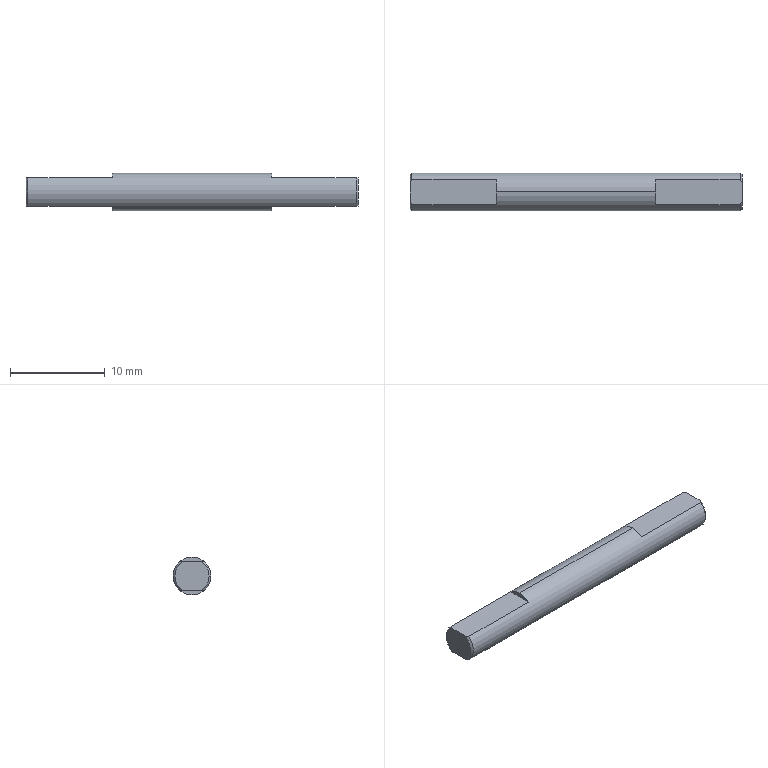Part | NX | features BREP 1 | 1 solid | 16 faces | box 35 x 4 x 4 mm | volume 406.634 mm3 | plane 10 | cone 4 | cylinder 2 | commonest cylinder face diameters 4 x2
STEP:
#1=CARTESIAN_POINT('',(34.8,1.323,-1.5));
#2=VERTEX_POINT('',#1);
#3=CARTESIAN_POINT('',(35.,0.995,-1.5));
#4=VERTEX_POINT('',#3);
#5=CARTESIAN_POINT('',(34.8,1.323,-1.5));
#6=CARTESIAN_POINT('',(34.876,1.208,-1.5));
#7=CARTESIAN_POINT('',(34.943,1.099,-1.5));
#8=CARTESIAN_POINT('',(35.,0.995,-1.5));
#9=B_SPLINE_CURVE_WITH_KNOTS('',3,(#5,#6,#7,#8),.UNSPECIFIED.,.F.,.F.,(4,4),(0.,1.),.UNSPECIFIED.);
#10=EDGE_CURVE('',#2,#4,#9,.T.);
#11=ORIENTED_EDGE('',*,*,#10,.F.);
#12=CARTESIAN_POINT('',(34.8,1.323,1.5));
#13=VERTEX_POINT('',#12);
#14=CARTESIAN_POINT('',(34.8,0.,0.));
#15=DIRECTION('',(-1.,0.,0.));
#16=DIRECTION('',(0.,0.,-1.));
#17=AXIS2_PLACEMENT_3D('',#14,#15,#16);
#18=CIRCLE('',#17,2.);
#19=EDGE_CURVE('',#13,#2,#18,.T.);
#20=ORIENTED_EDGE('',*,*,#19,.F.);
#21=CARTESIAN_POINT('',(35.,0.995,1.5));
#22=VERTEX_POINT('',#21);
#23=CARTESIAN_POINT('',(35.,0.995,1.5));
#24=CARTESIAN_POINT('',(34.943,1.099,1.5));
#25=CARTESIAN_POINT('',(34.876,1.208,1.5));
#26=CARTESIAN_POINT('',(34.8,1.323,1.5));
#27=B_SPLINE_CURVE_WITH_KNOTS('',3,(#23,#24,#25,#26),.UNSPECIFIED.,.F.,.F.,(4,4),(0.,1.),.UNSPECIFIED.);
#28=EDGE_CURVE('',#22,#13,#27,.T.);
#29=ORIENTED_EDGE('',*,*,#28,.F.);
#30=CARTESIAN_POINT('',(35.,0.,0.));
#31=DIRECTION('',(1.,0.,0.));
#32=DIRECTION('',(0.,0.,-1.));
#33=AXIS2_PLACEMENT_3D('',#30,#31,#32);
#34=CIRCLE('',#33,1.8);
#35=EDGE_CURVE('',#4,#22,#34,.T.);
#36=ORIENTED_EDGE('',*,*,#35,.F.);
#37=EDGE_LOOP('',(#11,#20,#29,#36));
#38=FACE_BOUND('',#37,.T.);
#39=CARTESIAN_POINT('',(35.,0.,0.));
#40=DIRECTION('',(-1.,0.,0.));
#41=DIRECTION('',(0.,0.,1.));
#42=AXIS2_PLACEMENT_3D('',#39,#40,#41);
#43=CONICAL_SURFACE('',#42,1.8,0.7854);
#44=ADVANCED_FACE('',(#38),#43,.T.);
#45=CARTESIAN_POINT('',(34.8,-1.323,1.5));
#46=VERTEX_POINT('',#45);
#47=CARTESIAN_POINT('',(35.,-0.995,1.5));
#48=VERTEX_POINT('',#47);
#49=CARTESIAN_POINT('',(34.8,-1.323,1.5));
#50=CARTESIAN_POINT('',(34.876,-1.208,1.5));
#51=CARTESIAN_POINT('',(34.943,-1.099,1.5));
#52=CARTESIAN_POINT('',(35.,-0.995,1.5));
#53=B_SPLINE_CURVE_WITH_KNOTS('',3,(#49,#50,#51,#52),.UNSPECIFIED.,.F.,.F.,(4,4),(0.,1.),.UNSPECIFIED.);
#54=EDGE_CURVE('',#46,#48,#53,.T.);
#55=ORIENTED_EDGE('',*,*,#54,.F.);
#56=CARTESIAN_POINT('',(34.8,-1.323,-1.5));
#57=VERTEX_POINT('',#56);
#58=CARTESIAN_POINT('',(34.8,0.,0.));
#59=DIRECTION('',(-1.,0.,0.));
#60=DIRECTION('',(0.,0.,-1.));
#61=AXIS2_PLACEMENT_3D('',#58,#59,#60);
#62=CIRCLE('',#61,2.);
#63=EDGE_CURVE('',#57,#46,#62,.T.);
#64=ORIENTED_EDGE('',*,*,#63,.F.);
#65=CARTESIAN_POINT('',(35.,-0.995,-1.5));
#66=VERTEX_POINT('',#65);
#67=CARTESIAN_POINT('',(35.,-0.995,-1.5));
#68=CARTESIAN_POINT('',(34.943,-1.099,-1.5));
#69=CARTESIAN_POINT('',(34.876,-1.208,-1.5));
#70=CARTESIAN_POINT('',(34.8,-1.323,-1.5));
#71=B_SPLINE_CURVE_WITH_KNOTS('',3,(#67,#68,#69,#70),.UNSPECIFIED.,.F.,.F.,(4,4),(0.,1.),.UNSPECIFIED.);
#72=EDGE_CURVE('',#66,#57,#71,.T.);
#73=ORIENTED_EDGE('',*,*,#72,.F.);
#74=CARTESIAN_POINT('',(35.,0.,0.));
#75=DIRECTION('',(1.,0.,0.));
#76=DIRECTION('',(0.,0.,-1.));
#77=AXIS2_PLACEMENT_3D('',#74,#75,#76);
#78=CIRCLE('',#77,1.8);
#79=EDGE_CURVE('',#48,#66,#78,.T.);
#80=ORIENTED_EDGE('',*,*,#79,.F.);
#81=EDGE_LOOP('',(#55,#64,#73,#80));
#82=FACE_BOUND('',#81,.T.);
#83=CARTESIAN_POINT('',(35.,0.,0.));
#84=DIRECTION('',(-1.,0.,0.));
#85=DIRECTION('',(0.,0.,1.));
#86=AXIS2_PLACEMENT_3D('',#83,#84,#85);
#87=CONICAL_SURFACE('',#86,1.8,0.7854);
#88=ADVANCED_FACE('',(#82),#87,.T.);
#89=CARTESIAN_POINT('',(0.,0.995,-1.5));
#90=VERTEX_POINT('',#89);
#91=CARTESIAN_POINT('',(0.2,1.323,-1.5));
#92=VERTEX_POINT('',#91);
#93=CARTESIAN_POINT('',(0.,0.995,-1.5));
#94=CARTESIAN_POINT('',(0.05724,1.099,-1.5));
#95=CARTESIAN_POINT('',(0.1239,1.208,-1.5));
#96=CARTESIAN_POINT('',(0.2,1.323,-1.5));
#97=B_SPLINE_CURVE_WITH_KNOTS('',3,(#93,#94,#95,#96),.UNSPECIFIED.,.F.,.F.,(4,4),(0.,1.),.UNSPECIFIED.);
#98=EDGE_CURVE('',#90,#92,#97,.T.);
#99=ORIENTED_EDGE('',*,*,#98,.F.);
#100=CARTESIAN_POINT('',(0.,0.995,1.5));
#101=VERTEX_POINT('',#100);
#102=CARTESIAN_POINT('',(0.,0.,0.));
#103=DIRECTION('',(-1.,0.,0.));
#104=DIRECTION('',(0.,0.,1.));
#105=AXIS2_PLACEMENT_3D('',#102,#103,#104);
#106=CIRCLE('',#105,1.8);
#107=EDGE_CURVE('',#101,#90,#106,.T.);
#108=ORIENTED_EDGE('',*,*,#107,.F.);
#109=CARTESIAN_POINT('',(0.2,1.323,1.5));
#110=VERTEX_POINT('',#109);
#111=CARTESIAN_POINT('',(0.2,1.323,1.5));
#112=CARTESIAN_POINT('',(0.1239,1.208,1.5));
#113=CARTESIAN_POINT('',(0.05724,1.099,1.5));
#114=CARTESIAN_POINT('',(0.,0.995,1.5));
#115=B_SPLINE_CURVE_WITH_KNOTS('',3,(#111,#112,#113,#114),.UNSPECIFIED.,.F.,.F.,(4,4),(0.,1.),.UNSPECIFIED.);
#116=EDGE_CURVE('',#110,#101,#115,.T.);
#117=ORIENTED_EDGE('',*,*,#116,.F.);
#118=CARTESIAN_POINT('',(0.2,0.,0.));
#119=DIRECTION('',(1.,0.,0.));
#120=DIRECTION('',(0.,0.,1.));
#121=AXIS2_PLACEMENT_3D('',#118,#119,#120);
#122=CIRCLE('',#121,2.);
#123=EDGE_CURVE('',#92,#110,#122,.T.);
#124=ORIENTED_EDGE('',*,*,#123,.F.);
#125=EDGE_LOOP('',(#99,#108,#117,#124));
#126=FACE_BOUND('',#125,.T.);
#127=CARTESIAN_POINT('',(0.2,0.,0.));
#128=DIRECTION('',(1.,0.,0.));
#129=DIRECTION('',(0.,0.,-1.));
#130=AXIS2_PLACEMENT_3D('',#127,#128,#129);
#131=CONICAL_SURFACE('',#130,2.,0.7854);
#132=ADVANCED_FACE('',(#126),#131,.T.);
#133=CARTESIAN_POINT('',(0.,-0.995,1.5));
#134=VERTEX_POINT('',#133);
#135=CARTESIAN_POINT('',(0.2,-1.323,1.5));
#136=VERTEX_POINT('',#135);
#137=CARTESIAN_POINT('',(0.,-0.995,1.5));
#138=CARTESIAN_POINT('',(0.05724,-1.099,1.5));
#139=CARTESIAN_POINT('',(0.1239,-1.208,1.5));
#140=CARTESIAN_POINT('',(0.2,-1.323,1.5));
#141=B_SPLINE_CURVE_WITH_KNOTS('',3,(#137,#138,#139,#140),.UNSPECIFIED.,.F.,.F.,(4,4),(0.,1.),.UNSPECIFIED.);
#142=EDGE_CURVE('',#134,#136,#141,.T.);
#143=ORIENTED_EDGE('',*,*,#142,.F.);
#144=CARTESIAN_POINT('',(0.,-0.995,-1.5));
#145=VERTEX_POINT('',#144);
#146=CARTESIAN_POINT('',(0.,0.,0.));
#147=DIRECTION('',(-1.,0.,0.));
#148=DIRECTION('',(0.,0.,1.));
#149=AXIS2_PLACEMENT_3D('',#146,#147,#148);
#150=CIRCLE('',#149,1.8);
#151=EDGE_CURVE('',#145,#134,#150,.T.);
#152=ORIENTED_EDGE('',*,*,#151,.F.);
#153=CARTESIAN_POINT('',(0.2,-1.323,-1.5));
#154=VERTEX_POINT('',#153);
#155=CARTESIAN_POINT('',(0.2,-1.323,-1.5));
#156=CARTESIAN_POINT('',(0.1239,-1.208,-1.5));
#157=CARTESIAN_POINT('',(0.05724,-1.099,-1.5));
#158=CARTESIAN_POINT('',(0.,-0.995,-1.5));
#159=B_SPLINE_CURVE_WITH_KNOTS('',3,(#155,#156,#157,#158),.UNSPECIFIED.,.F.,.F.,(4,4),(0.,1.),.UNSPECIFIED.);
#160=EDGE_CURVE('',#154,#145,#159,.T.);
#161=ORIENTED_EDGE('',*,*,#160,.F.);
#162=CARTESIAN_POINT('',(0.2,0.,0.));
#163=DIRECTION('',(1.,0.,0.));
#164=DIRECTION('',(0.,0.,1.));
#165=AXIS2_PLACEMENT_3D('',#162,#163,#164);
#166=CIRCLE('',#165,2.);
#167=EDGE_CURVE('',#136,#154,#166,.T.);
#168=ORIENTED_EDGE('',*,*,#167,.F.);
#169=EDGE_LOOP('',(#143,#152,#161,#168));
#170=FACE_BOUND('',#169,.T.);
#171=CARTESIAN_POINT('',(0.2,0.,0.));
#172=DIRECTION('',(1.,0.,0.));
#173=DIRECTION('',(0.,0.,-1.));
#174=AXIS2_PLACEMENT_3D('',#171,#172,#173);
#175=CONICAL_SURFACE('',#174,2.,0.7854);
#176=ADVANCED_FACE('',(#170),#175,.T.);
#177=CARTESIAN_POINT('',(9.1,-1.323,-1.5));
#178=VERTEX_POINT('',#177);
#179=CARTESIAN_POINT('',(0.,-1.323,-1.5));
#180=DIRECTION('',(-1.,0.,0.));
#181=VECTOR('',#180,1000.);
#182=LINE('',#179,#181);
#183=EDGE_CURVE('',#178,#154,#182,.T.);
#184=ORIENTED_EDGE('',*,*,#183,.T.);
#185=ORIENTED_EDGE('',*,*,#160,.T.);
#186=CARTESIAN_POINT('',(0.,0.,-1.5));
#187=DIRECTION('',(0.,1.,0.));
#188=VECTOR('',#187,1000.);
#189=LINE('',#186,#188);
#190=EDGE_CURVE('',#145,#90,#189,.T.);
#191=ORIENTED_EDGE('',*,*,#190,.T.);
#192=ORIENTED_EDGE('',*,*,#98,.T.);
#193=CARTESIAN_POINT('',(9.1,1.323,-1.5));
#194=VERTEX_POINT('',#193);
#195=CARTESIAN_POINT('',(0.,1.323,-1.5));
#196=DIRECTION('',(1.,0.,0.));
#197=VECTOR('',#196,1000.);
#198=LINE('',#195,#197);
#199=EDGE_CURVE('',#92,#194,#198,.T.);
#200=ORIENTED_EDGE('',*,*,#199,.T.);
#201=CARTESIAN_POINT('',(9.1,-2.,-1.5));
#202=DIRECTION('',(0.,1.,0.));
#203=VECTOR('',#202,1000.);
#204=LINE('',#201,#203);
#205=EDGE_CURVE('',#178,#194,#204,.T.);
#206=ORIENTED_EDGE('',*,*,#205,.F.);
#207=EDGE_LOOP('',(#184,#185,#191,#192,#200,#206));
#208=FACE_BOUND('',#207,.T.);
#209=CARTESIAN_POINT('',(9.1,-2.,-1.5));
#210=DIRECTION('',(0.,0.,1.));
#211=DIRECTION('',(1.,0.,0.));
#212=AXIS2_PLACEMENT_3D('',#209,#210,#211);
#213=PLANE('',#212);
#214=ADVANCED_FACE('',(#208),#213,.F.);
#215=CARTESIAN_POINT('',(9.1,0.,-2.));
#216=VERTEX_POINT('',#215);
#217=CARTESIAN_POINT('',(9.1,0.,0.));
#218=DIRECTION('',(-1.,0.,0.));
#219=DIRECTION('',(0.,0.,-1.));
#220=AXIS2_PLACEMENT_3D('',#217,#218,#219);
#221=CIRCLE('',#220,2.);
#222=EDGE_CURVE('',#194,#216,#221,.T.);
#223=ORIENTED_EDGE('',*,*,#222,.T.);
#224=CARTESIAN_POINT('',(9.1,0.,0.));
#225=DIRECTION('',(-1.,0.,0.));
#226=DIRECTION('',(0.,0.,-1.));
#227=AXIS2_PLACEMENT_3D('',#224,#225,#226);
#228=CIRCLE('',#227,2.);
#229=EDGE_CURVE('',#216,#178,#228,.T.);
#230=ORIENTED_EDGE('',*,*,#229,.T.);
#231=ORIENTED_EDGE('',*,*,#205,.T.);
#232=EDGE_LOOP('',(#223,#230,#231));
#233=FACE_BOUND('',#232,.T.);
#234=CARTESIAN_POINT('',(9.1,0.,0.));
#235=DIRECTION('',(1.,0.,0.));
#236=DIRECTION('',(0.,0.,-1.));
#237=AXIS2_PLACEMENT_3D('',#234,#235,#236);
#238=PLANE('',#237);
#239=ADVANCED_FACE('',(#233),#238,.F.);
#240=CARTESIAN_POINT('',(9.1,-1.323,1.5));
#241=VERTEX_POINT('',#240);
#242=CARTESIAN_POINT('',(9.1,0.,2.));
#243=VERTEX_POINT('',#242);
#244=CARTESIAN_POINT('',(9.1,0.,0.));
#245=DIRECTION('',(-1.,0.,0.));
#246=DIRECTION('',(0.,0.,-1.));
#247=AXIS2_PLACEMENT_3D('',#244,#245,#246);
#248=CIRCLE('',#247,2.);
#249=EDGE_CURVE('',#241,#243,#248,.T.);
#250=ORIENTED_EDGE('',*,*,#249,.T.);
#251=CARTESIAN_POINT('',(9.1,1.323,1.5));
#252=VERTEX_POINT('',#251);
#253=CARTESIAN_POINT('',(9.1,0.,0.));
#254=DIRECTION('',(-1.,0.,0.));
#255=DIRECTION('',(0.,0.,-1.));
#256=AXIS2_PLACEMENT_3D('',#253,#254,#255);
#257=CIRCLE('',#256,2.);
#258=EDGE_CURVE('',#243,#252,#257,.T.);
#259=ORIENTED_EDGE('',*,*,#258,.T.);
#260=CARTESIAN_POINT('',(9.1,-2.,1.5));
#261=DIRECTION('',(0.,-1.,0.));
#262=VECTOR('',#261,1000.);
#263=LINE('',#260,#262);
#264=EDGE_CURVE('',#252,#241,#263,.T.);
#265=ORIENTED_EDGE('',*,*,#264,.T.);
#266=EDGE_LOOP('',(#250,#259,#265));
#267=FACE_BOUND('',#266,.T.);
#268=CARTESIAN_POINT('',(9.1,0.,0.));
#269=DIRECTION('',(1.,0.,0.));
#270=DIRECTION('',(0.,0.,-1.));
#271=AXIS2_PLACEMENT_3D('',#268,#269,#270);
#272=PLANE('',#271);
#273=ADVANCED_FACE('',(#267),#272,.F.);
#274=CARTESIAN_POINT('',(0.,0.,1.5));
#275=DIRECTION('',(0.,-1.,0.));
#276=VECTOR('',#275,1000.);
#277=LINE('',#274,#276);
#278=EDGE_CURVE('',#101,#134,#277,.T.);
#279=ORIENTED_EDGE('',*,*,#278,.T.);
#280=ORIENTED_EDGE('',*,*,#142,.T.);
#281=CARTESIAN_POINT('',(0.,-1.323,1.5));
#282=DIRECTION('',(1.,0.,0.));
#283=VECTOR('',#282,1000.);
#284=LINE('',#281,#283);
#285=EDGE_CURVE('',#136,#241,#284,.T.);
#286=ORIENTED_EDGE('',*,*,#285,.T.);
#287=ORIENTED_EDGE('',*,*,#264,.F.);
#288=CARTESIAN_POINT('',(0.,1.323,1.5));
#289=DIRECTION('',(-1.,0.,0.));
#290=VECTOR('',#289,1000.);
#291=LINE('',#288,#290);
#292=EDGE_CURVE('',#252,#110,#291,.T.);
#293=ORIENTED_EDGE('',*,*,#292,.T.);
#294=ORIENTED_EDGE('',*,*,#116,.T.);
#295=EDGE_LOOP('',(#279,#280,#286,#287,#293,#294));
#296=FACE_BOUND('',#295,.T.);
#297=CARTESIAN_POINT('',(9.1,-2.,1.5));
#298=DIRECTION('',(0.,0.,-1.));
#299=DIRECTION('',(-1.,0.,0.));
#300=AXIS2_PLACEMENT_3D('',#297,#298,#299);
#301=PLANE('',#300);
#302=ADVANCED_FACE('',(#296),#301,.F.);
#303=CARTESIAN_POINT('',(35.,0.,-1.5));
#304=DIRECTION('',(0.,1.,0.));
#305=VECTOR('',#304,1000.);
#306=LINE('',#303,#305);
#307=EDGE_CURVE('',#66,#4,#306,.T.);
#308=ORIENTED_EDGE('',*,*,#307,.F.);
#309=ORIENTED_EDGE('',*,*,#72,.T.);
#310=CARTESIAN_POINT('',(25.9,-1.323,-1.5));
#311=VERTEX_POINT('',#310);
#312=CARTESIAN_POINT('',(0.,-1.323,-1.5));
#313=DIRECTION('',(1.,0.,0.));
#314=VECTOR('',#313,1000.);
#315=LINE('',#312,#314);
#316=EDGE_CURVE('',#311,#57,#315,.T.);
#317=ORIENTED_EDGE('',*,*,#316,.F.);
#318=CARTESIAN_POINT('',(25.9,1.323,-1.5));
#319=VERTEX_POINT('',#318);
#320=CARTESIAN_POINT('',(25.9,-2.,-1.5));
#321=DIRECTION('',(0.,1.,0.));
#322=VECTOR('',#321,1000.);
#323=LINE('',#320,#322);
#324=EDGE_CURVE('',#311,#319,#323,.T.);
#325=ORIENTED_EDGE('',*,*,#324,.T.);
#326=CARTESIAN_POINT('',(0.,1.323,-1.5));
#327=DIRECTION('',(-1.,0.,0.));
#328=VECTOR('',#327,1000.);
#329=LINE('',#326,#328);
#330=EDGE_CURVE('',#2,#319,#329,.T.);
#331=ORIENTED_EDGE('',*,*,#330,.F.);
#332=ORIENTED_EDGE('',*,*,#10,.T.);
#333=EDGE_LOOP('',(#308,#309,#317,#325,#331,#332));
#334=FACE_BOUND('',#333,.T.);
#335=CARTESIAN_POINT('',(25.9,-2.,-1.5));
#336=DIRECTION('',(0.,0.,-1.));
#337=DIRECTION('',(-1.,0.,0.));
#338=AXIS2_PLACEMENT_3D('',#335,#336,#337);
#339=PLANE('',#338);
#340=ADVANCED_FACE('',(#334),#339,.T.);
#341=ORIENTED_EDGE('',*,*,#324,.F.);
#342=CARTESIAN_POINT('',(25.9,0.,-2.));
#343=VERTEX_POINT('',#342);
#344=CARTESIAN_POINT('',(25.9,0.,0.));
#345=DIRECTION('',(-1.,0.,0.));
#346=DIRECTION('',(0.,0.,-1.));
#347=AXIS2_PLACEMENT_3D('',#344,#345,#346);
#348=CIRCLE('',#347,2.);
#349=EDGE_CURVE('',#343,#311,#348,.T.);
#350=ORIENTED_EDGE('',*,*,#349,.F.);
#351=CARTESIAN_POINT('',(25.9,0.,0.));
#352=DIRECTION('',(-1.,0.,0.));
#353=DIRECTION('',(0.,0.,-1.));
#354=AXIS2_PLACEMENT_3D('',#351,#352,#353);
#355=CIRCLE('',#354,2.);
#356=EDGE_CURVE('',#319,#343,#355,.T.);
#357=ORIENTED_EDGE('',*,*,#356,.F.);
#358=EDGE_LOOP('',(#341,#350,#357));
#359=FACE_BOUND('',#358,.T.);
#360=CARTESIAN_POINT('',(25.9,0.,0.));
#361=DIRECTION('',(1.,0.,0.));
#362=DIRECTION('',(0.,0.,-1.));
#363=AXIS2_PLACEMENT_3D('',#360,#361,#362);
#364=PLANE('',#363);
#365=ADVANCED_FACE('',(#359),#364,.T.);
#366=CARTESIAN_POINT('',(25.9,1.323,1.5));
#367=VERTEX_POINT('',#366);
#368=CARTESIAN_POINT('',(25.9,-1.323,1.5));
#369=VERTEX_POINT('',#368);
#370=CARTESIAN_POINT('',(25.9,-2.,1.5));
#371=DIRECTION('',(0.,-1.,0.));
#372=VECTOR('',#371,1000.);
#373=LINE('',#370,#372);
#374=EDGE_CURVE('',#367,#369,#373,.T.);
#375=ORIENTED_EDGE('',*,*,#374,.F.);
#376=CARTESIAN_POINT('',(25.9,0.,2.));
#377=VERTEX_POINT('',#376);
#378=CARTESIAN_POINT('',(25.9,0.,0.));
#379=DIRECTION('',(-1.,0.,0.));
#380=DIRECTION('',(0.,0.,-1.));
#381=AXIS2_PLACEMENT_3D('',#378,#379,#380);
#382=CIRCLE('',#381,2.);
#383=EDGE_CURVE('',#377,#367,#382,.T.);
#384=ORIENTED_EDGE('',*,*,#383,.F.);
#385=CARTESIAN_POINT('',(25.9,0.,0.));
#386=DIRECTION('',(-1.,0.,0.));
#387=DIRECTION('',(0.,0.,-1.));
#388=AXIS2_PLACEMENT_3D('',#385,#386,#387);
#389=CIRCLE('',#388,2.);
#390=EDGE_CURVE('',#369,#377,#389,.T.);
#391=ORIENTED_EDGE('',*,*,#390,.F.);
#392=EDGE_LOOP('',(#375,#384,#391));
#393=FACE_BOUND('',#392,.T.);
#394=CARTESIAN_POINT('',(25.9,0.,0.));
#395=DIRECTION('',(1.,0.,0.));
#396=DIRECTION('',(0.,0.,-1.));
#397=AXIS2_PLACEMENT_3D('',#394,#395,#396);
#398=PLANE('',#397);
#399=ADVANCED_FACE('',(#393),#398,.T.);
#400=CARTESIAN_POINT('',(0.,-1.323,1.5));
#401=DIRECTION('',(-1.,0.,0.));
#402=VECTOR('',#401,1000.);
#403=LINE('',#400,#402);
#404=EDGE_CURVE('',#46,#369,#403,.T.);
#405=ORIENTED_EDGE('',*,*,#404,.F.);
#406=ORIENTED_EDGE('',*,*,#54,.T.);
#407=CARTESIAN_POINT('',(35.,0.,1.5));
#408=DIRECTION('',(0.,-1.,0.));
#409=VECTOR('',#408,1000.);
#410=LINE('',#407,#409);
#411=EDGE_CURVE('',#22,#48,#410,.T.);
#412=ORIENTED_EDGE('',*,*,#411,.F.);
#413=ORIENTED_EDGE('',*,*,#28,.T.);
#414=CARTESIAN_POINT('',(0.,1.323,1.5));
#415=DIRECTION('',(1.,0.,0.));
#416=VECTOR('',#415,1000.);
#417=LINE('',#414,#416);
#418=EDGE_CURVE('',#367,#13,#417,.T.);
#419=ORIENTED_EDGE('',*,*,#418,.F.);
#420=ORIENTED_EDGE('',*,*,#374,.T.);
#421=EDGE_LOOP('',(#405,#406,#412,#413,#419,#420));
#422=FACE_BOUND('',#421,.T.);
#423=CARTESIAN_POINT('',(25.9,-2.,1.5));
#424=DIRECTION('',(0.,0.,1.));
#425=DIRECTION('',(1.,0.,0.));
#426=AXIS2_PLACEMENT_3D('',#423,#424,#425);
#427=PLANE('',#426);
#428=ADVANCED_FACE('',(#422),#427,.T.);
#429=ORIENTED_EDGE('',*,*,#190,.F.);
#430=ORIENTED_EDGE('',*,*,#151,.T.);
#431=ORIENTED_EDGE('',*,*,#278,.F.);
#432=ORIENTED_EDGE('',*,*,#107,.T.);
#433=EDGE_LOOP('',(#429,#430,#431,#432));
#434=FACE_BOUND('',#433,.T.);
#435=CARTESIAN_POINT('',(0.,0.,0.));
#436=DIRECTION('',(-1.,0.,0.));
#437=DIRECTION('',(0.,0.,1.));
#438=AXIS2_PLACEMENT_3D('',#435,#436,#437);
#439=PLANE('',#438);
#440=ADVANCED_FACE('',(#434),#439,.T.);
#441=ORIENTED_EDGE('',*,*,#411,.T.);
#442=ORIENTED_EDGE('',*,*,#79,.T.);
#443=ORIENTED_EDGE('',*,*,#307,.T.);
#444=ORIENTED_EDGE('',*,*,#35,.T.);
#445=EDGE_LOOP('',(#441,#442,#443,#444));
#446=FACE_BOUND('',#445,.T.);
#447=CARTESIAN_POINT('',(35.,0.,0.));
#448=DIRECTION('',(1.,0.,0.));
#449=DIRECTION('',(0.,0.,-1.));
#450=AXIS2_PLACEMENT_3D('',#447,#448,#449);
#451=PLANE('',#450);
#452=ADVANCED_FACE('',(#446),#451,.T.);
#453=CARTESIAN_POINT('',(0.,0.,2.));
#454=DIRECTION('',(1.,0.,0.));
#455=VECTOR('',#454,1000.);
#456=LINE('',#453,#455);
#457=EDGE_CURVE('',#243,#377,#456,.T.);
#458=ORIENTED_EDGE('',*,*,#457,.F.);
#459=ORIENTED_EDGE('',*,*,#249,.F.);
#460=ORIENTED_EDGE('',*,*,#285,.F.);
#461=ORIENTED_EDGE('',*,*,#167,.T.);
#462=ORIENTED_EDGE('',*,*,#183,.F.);
#463=ORIENTED_EDGE('',*,*,#229,.F.);
#464=CARTESIAN_POINT('',(0.,0.,-2.));
#465=DIRECTION('',(1.,0.,0.));
#466=VECTOR('',#465,1000.);
#467=LINE('',#464,#466);
#468=EDGE_CURVE('',#216,#343,#467,.T.);
#469=ORIENTED_EDGE('',*,*,#468,.T.);
#470=ORIENTED_EDGE('',*,*,#349,.T.);
#471=ORIENTED_EDGE('',*,*,#316,.T.);
#472=ORIENTED_EDGE('',*,*,#63,.T.);
#473=ORIENTED_EDGE('',*,*,#404,.T.);
#474=ORIENTED_EDGE('',*,*,#390,.T.);
#475=EDGE_LOOP('',(#458,#459,#460,#461,#462,#463,#469,#470,#471,#472,#473,#474));
#476=FACE_BOUND('',#475,.T.);
#477=CARTESIAN_POINT('',(0.,0.,0.));
#478=DIRECTION('',(1.,0.,0.));
#479=DIRECTION('',(0.,0.,-1.));
#480=AXIS2_PLACEMENT_3D('',#477,#478,#479);
#481=CYLINDRICAL_SURFACE('',#480,2.);
#482=ADVANCED_FACE('',(#476),#481,.T.);
#483=ORIENTED_EDGE('',*,*,#258,.F.);
#484=ORIENTED_EDGE('',*,*,#457,.T.);
#485=ORIENTED_EDGE('',*,*,#383,.T.);
#486=ORIENTED_EDGE('',*,*,#418,.T.);
#487=ORIENTED_EDGE('',*,*,#19,.T.);
#488=ORIENTED_EDGE('',*,*,#330,.T.);
#489=ORIENTED_EDGE('',*,*,#356,.T.);
#490=ORIENTED_EDGE('',*,*,#468,.F.);
#491=ORIENTED_EDGE('',*,*,#222,.F.);
#492=ORIENTED_EDGE('',*,*,#199,.F.);
#493=ORIENTED_EDGE('',*,*,#123,.T.);
#494=ORIENTED_EDGE('',*,*,#292,.F.);
#495=EDGE_LOOP('',(#483,#484,#485,#486,#487,#488,#489,#490,#491,#492,#493,#494));
#496=FACE_BOUND('',#495,.T.);
#497=CARTESIAN_POINT('',(0.,0.,0.));
#498=DIRECTION('',(1.,0.,0.));
#499=DIRECTION('',(0.,0.,-1.));
#500=AXIS2_PLACEMENT_3D('',#497,#498,#499);
#501=CYLINDRICAL_SURFACE('',#500,2.);
#502=ADVANCED_FACE('',(#496),#501,.T.);
#503=CLOSED_SHELL('',(#44,#88,#132,#176,#214,#239,#273,#302,#340,#365,#399,#428,#440,#452,#482,#502));
#504=MANIFOLD_SOLID_BREP('',#503);
#505=(LENGTH_UNIT()NAMED_UNIT(*)SI_UNIT(.MILLI.,.METRE.));
#506=UNCERTAINTY_MEASURE_WITH_UNIT(LENGTH_MEASURE(0.0508),#505,'','');
#507=(NAMED_UNIT(*)PLANE_ANGLE_UNIT()SI_UNIT($,.RADIAN.));
#508=(NAMED_UNIT(*)SI_UNIT($,.STERADIAN.)SOLID_ANGLE_UNIT());
#509=(GEOMETRIC_REPRESENTATION_CONTEXT(3)GLOBAL_UNCERTAINTY_ASSIGNED_CONTEXT((#506))GLOBAL_UNIT_ASSIGNED_CONTEXT((#505,#507,#508))REPRESENTATION_CONTEXT('',''));
#510=ADVANCED_BREP_SHAPE_REPRESENTATION('',(#504),#509);